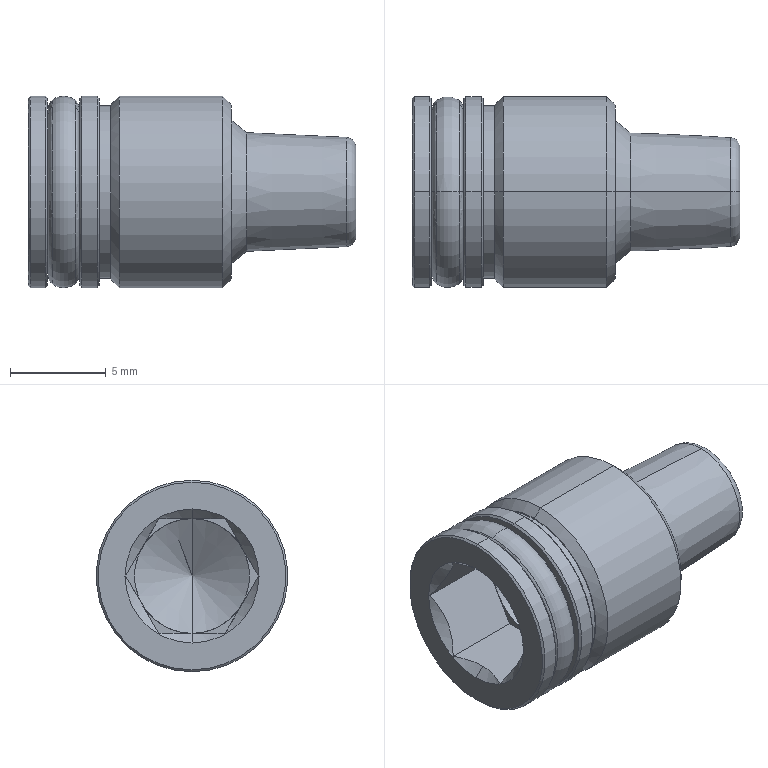Part | STEP file | 63_C_Screw | 1 solid | 65 faces | box 17.1 x 10 x 10 mm | volume 818.333 mm3 | cone 20 | plane 19 | cylinder 14 | torus 12 | commonest cylinder face diameters 10 x6 7.7 x4 6 x2 9 x2